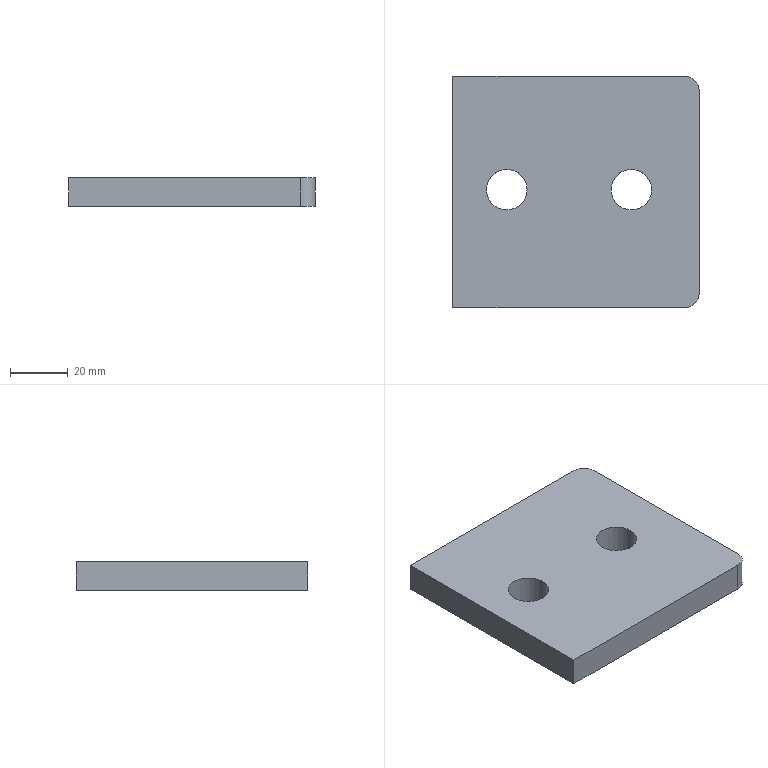Part | SolidWorks | features Extrusion 1, HoleWzd 1 | 1 solid | 12 faces | box 85 x 80 x 10 mm | volume 64814 mm3 | cylinder 6 | plane 6 | commonest cylinder face diameters 14 x4 10 x2
STEP:
#1=CARTESIAN_POINT('',(12.1,0.8,0.));
#2=VERTEX_POINT('',#1);
#3=CARTESIAN_POINT('',(26.1,0.8,0.));
#4=VERTEX_POINT('',#3);
#5=CARTESIAN_POINT('',(19.1,0.8,0.));
#6=DIRECTION('',(0.,0.,1.));
#7=DIRECTION('',(1.,0.,0.));
#8=AXIS2_PLACEMENT_3D('',#5,#6,#7);
#9=CIRCLE('',#8,7.);
#10=EDGE_CURVE('',#2,#4,#9,.T.);
#11=ORIENTED_EDGE('',*,*,#10,.F.);
#12=CARTESIAN_POINT('',(12.1,0.8,10.));
#13=VERTEX_POINT('',#12);
#14=CARTESIAN_POINT('',(12.1,0.8,10.));
#15=DIRECTION('',(0.,0.,1.));
#16=VECTOR('',#15,1000.);
#17=LINE('',#14,#16);
#18=EDGE_CURVE('',#2,#13,#17,.T.);
#19=ORIENTED_EDGE('',*,*,#18,.T.);
#20=CARTESIAN_POINT('',(26.1,0.8,10.));
#21=VERTEX_POINT('',#20);
#22=CARTESIAN_POINT('',(19.1,0.8,10.));
#23=DIRECTION('',(0.,0.,1.));
#24=DIRECTION('',(1.,0.,0.));
#25=AXIS2_PLACEMENT_3D('',#22,#23,#24);
#26=CIRCLE('',#25,7.);
#27=EDGE_CURVE('',#13,#21,#26,.T.);
#28=ORIENTED_EDGE('',*,*,#27,.T.);
#29=CARTESIAN_POINT('',(26.1,0.8,10.));
#30=DIRECTION('',(0.,0.,1.));
#31=VECTOR('',#30,1000.);
#32=LINE('',#29,#31);
#33=EDGE_CURVE('',#4,#21,#32,.T.);
#34=ORIENTED_EDGE('',*,*,#33,.F.);
#35=EDGE_LOOP('',(#11,#19,#28,#34));
#36=FACE_OUTER_BOUND('',#35,.T.);
#37=CARTESIAN_POINT('',(19.1,0.8,10.));
#38=DIRECTION('',(0.,0.,1.));
#39=DIRECTION('',(1.,0.,0.));
#40=AXIS2_PLACEMENT_3D('',#37,#38,#39);
#41=CYLINDRICAL_SURFACE('',#40,7.);
#42=ADVANCED_FACE('',(#36),#41,.F.);
#43=CARTESIAN_POINT('',(-30.9,0.8,0.));
#44=VERTEX_POINT('',#43);
#45=CARTESIAN_POINT('',(-16.9,0.8,0.));
#46=VERTEX_POINT('',#45);
#47=CARTESIAN_POINT('',(-23.9,0.8,0.));
#48=DIRECTION('',(0.,0.,1.));
#49=DIRECTION('',(1.,0.,0.));
#50=AXIS2_PLACEMENT_3D('',#47,#48,#49);
#51=CIRCLE('',#50,7.);
#52=EDGE_CURVE('',#44,#46,#51,.T.);
#53=ORIENTED_EDGE('',*,*,#52,.F.);
#54=CARTESIAN_POINT('',(-30.9,0.8,10.));
#55=VERTEX_POINT('',#54);
#56=CARTESIAN_POINT('',(-30.9,0.8,10.));
#57=DIRECTION('',(0.,0.,1.));
#58=VECTOR('',#57,1000.);
#59=LINE('',#56,#58);
#60=EDGE_CURVE('',#44,#55,#59,.T.);
#61=ORIENTED_EDGE('',*,*,#60,.T.);
#62=CARTESIAN_POINT('',(-16.9,0.8,10.));
#63=VERTEX_POINT('',#62);
#64=CARTESIAN_POINT('',(-23.9,0.8,10.));
#65=DIRECTION('',(0.,0.,1.));
#66=DIRECTION('',(1.,0.,0.));
#67=AXIS2_PLACEMENT_3D('',#64,#65,#66);
#68=CIRCLE('',#67,7.);
#69=EDGE_CURVE('',#55,#63,#68,.T.);
#70=ORIENTED_EDGE('',*,*,#69,.T.);
#71=CARTESIAN_POINT('',(-16.9,0.8,10.));
#72=DIRECTION('',(0.,0.,1.));
#73=VECTOR('',#72,1000.);
#74=LINE('',#71,#73);
#75=EDGE_CURVE('',#46,#63,#74,.T.);
#76=ORIENTED_EDGE('',*,*,#75,.F.);
#77=EDGE_LOOP('',(#53,#61,#70,#76));
#78=FACE_OUTER_BOUND('',#77,.T.);
#79=CARTESIAN_POINT('',(-23.9,0.8,10.));
#80=DIRECTION('',(0.,0.,1.));
#81=DIRECTION('',(1.,0.,0.));
#82=AXIS2_PLACEMENT_3D('',#79,#80,#81);
#83=CYLINDRICAL_SURFACE('',#82,7.);
#84=ADVANCED_FACE('',(#78),#83,.F.);
#85=CARTESIAN_POINT('',(-42.5,40.,0.));
#86=VERTEX_POINT('',#85);
#87=CARTESIAN_POINT('',(-42.5,-40.,0.));
#88=VERTEX_POINT('',#87);
#89=CARTESIAN_POINT('',(-42.5,40.,0.));
#90=DIRECTION('',(0.,-1.,0.));
#91=VECTOR('',#90,1000.);
#92=LINE('',#89,#91);
#93=EDGE_CURVE('',#86,#88,#92,.T.);
#94=ORIENTED_EDGE('',*,*,#93,.T.);
#95=CARTESIAN_POINT('',(-42.5,-40.,10.));
#96=VERTEX_POINT('',#95);
#97=CARTESIAN_POINT('',(-42.5,-40.,10.));
#98=DIRECTION('',(0.,0.,-1.));
#99=VECTOR('',#98,1000.);
#100=LINE('',#97,#99);
#101=EDGE_CURVE('',#96,#88,#100,.T.);
#102=ORIENTED_EDGE('',*,*,#101,.F.);
#103=CARTESIAN_POINT('',(-42.5,40.,10.));
#104=VERTEX_POINT('',#103);
#105=CARTESIAN_POINT('',(-42.5,40.,10.));
#106=DIRECTION('',(0.,-1.,0.));
#107=VECTOR('',#106,1000.);
#108=LINE('',#105,#107);
#109=EDGE_CURVE('',#104,#96,#108,.T.);
#110=ORIENTED_EDGE('',*,*,#109,.F.);
#111=CARTESIAN_POINT('',(-42.5,40.,10.));
#112=DIRECTION('',(0.,0.,-1.));
#113=VECTOR('',#112,1000.);
#114=LINE('',#111,#113);
#115=EDGE_CURVE('',#104,#86,#114,.T.);
#116=ORIENTED_EDGE('',*,*,#115,.T.);
#117=EDGE_LOOP('',(#94,#102,#110,#116));
#118=FACE_OUTER_BOUND('',#117,.T.);
#119=CARTESIAN_POINT('',(-42.5,40.,10.));
#120=DIRECTION('',(1.,0.,0.));
#121=DIRECTION('',(0.,1.,0.));
#122=AXIS2_PLACEMENT_3D('',#119,#120,#121);
#123=PLANE('',#122);
#124=ADVANCED_FACE('',(#118),#123,.F.);
#125=CARTESIAN_POINT('',(37.5,-40.,0.));
#126=VERTEX_POINT('',#125);
#127=CARTESIAN_POINT('',(-42.5,-40.,0.));
#128=DIRECTION('',(1.,0.,0.));
#129=VECTOR('',#128,1000.);
#130=LINE('',#127,#129);
#131=EDGE_CURVE('',#88,#126,#130,.T.);
#132=ORIENTED_EDGE('',*,*,#131,.T.);
#133=CARTESIAN_POINT('',(37.5,-40.,10.));
#134=VERTEX_POINT('',#133);
#135=CARTESIAN_POINT('',(37.5,-40.,10.));
#136=DIRECTION('',(0.,0.,-1.));
#137=VECTOR('',#136,1000.);
#138=LINE('',#135,#137);
#139=EDGE_CURVE('',#134,#126,#138,.T.);
#140=ORIENTED_EDGE('',*,*,#139,.F.);
#141=CARTESIAN_POINT('',(-42.5,-40.,10.));
#142=DIRECTION('',(1.,0.,0.));
#143=VECTOR('',#142,1000.);
#144=LINE('',#141,#143);
#145=EDGE_CURVE('',#96,#134,#144,.T.);
#146=ORIENTED_EDGE('',*,*,#145,.F.);
#147=ORIENTED_EDGE('',*,*,#101,.T.);
#148=EDGE_LOOP('',(#132,#140,#146,#147));
#149=FACE_OUTER_BOUND('',#148,.T.);
#150=CARTESIAN_POINT('',(-42.5,-40.,10.));
#151=DIRECTION('',(0.,1.,0.));
#152=DIRECTION('',(0.,0.,1.));
#153=AXIS2_PLACEMENT_3D('',#150,#151,#152);
#154=PLANE('',#153);
#155=ADVANCED_FACE('',(#149),#154,.F.);
#156=CARTESIAN_POINT('',(42.5,-35.,0.));
#157=VERTEX_POINT('',#156);
#158=CARTESIAN_POINT('',(37.5,-35.,0.));
#159=DIRECTION('',(0.,0.,1.));
#160=DIRECTION('',(1.,0.,0.));
#161=AXIS2_PLACEMENT_3D('',#158,#159,#160);
#162=CIRCLE('',#161,5.);
#163=EDGE_CURVE('',#126,#157,#162,.T.);
#164=ORIENTED_EDGE('',*,*,#163,.T.);
#165=CARTESIAN_POINT('',(42.5,-35.,10.));
#166=VERTEX_POINT('',#165);
#167=CARTESIAN_POINT('',(42.5,-35.,10.));
#168=DIRECTION('',(0.,0.,-1.));
#169=VECTOR('',#168,1000.);
#170=LINE('',#167,#169);
#171=EDGE_CURVE('',#166,#157,#170,.T.);
#172=ORIENTED_EDGE('',*,*,#171,.F.);
#173=CARTESIAN_POINT('',(37.5,-35.,10.));
#174=DIRECTION('',(0.,0.,1.));
#175=DIRECTION('',(1.,0.,0.));
#176=AXIS2_PLACEMENT_3D('',#173,#174,#175);
#177=CIRCLE('',#176,5.);
#178=EDGE_CURVE('',#134,#166,#177,.T.);
#179=ORIENTED_EDGE('',*,*,#178,.F.);
#180=ORIENTED_EDGE('',*,*,#139,.T.);
#181=EDGE_LOOP('',(#164,#172,#179,#180));
#182=FACE_OUTER_BOUND('',#181,.T.);
#183=CARTESIAN_POINT('',(37.5,-35.,10.));
#184=DIRECTION('',(0.,0.,-1.));
#185=DIRECTION('',(-1.,0.,0.));
#186=AXIS2_PLACEMENT_3D('',#183,#184,#185);
#187=CYLINDRICAL_SURFACE('',#186,5.);
#188=ADVANCED_FACE('',(#182),#187,.T.);
#189=CARTESIAN_POINT('',(42.5,35.,0.));
#190=VERTEX_POINT('',#189);
#191=CARTESIAN_POINT('',(42.5,35.,0.));
#192=DIRECTION('',(0.,1.,0.));
#193=VECTOR('',#192,1000.);
#194=LINE('',#191,#193);
#195=EDGE_CURVE('',#157,#190,#194,.T.);
#196=ORIENTED_EDGE('',*,*,#195,.T.);
#197=CARTESIAN_POINT('',(42.5,35.,10.));
#198=VERTEX_POINT('',#197);
#199=CARTESIAN_POINT('',(42.5,35.,10.));
#200=DIRECTION('',(0.,0.,-1.));
#201=VECTOR('',#200,1000.);
#202=LINE('',#199,#201);
#203=EDGE_CURVE('',#198,#190,#202,.T.);
#204=ORIENTED_EDGE('',*,*,#203,.F.);
#205=CARTESIAN_POINT('',(42.5,35.,10.));
#206=DIRECTION('',(0.,1.,0.));
#207=VECTOR('',#206,1000.);
#208=LINE('',#205,#207);
#209=EDGE_CURVE('',#166,#198,#208,.T.);
#210=ORIENTED_EDGE('',*,*,#209,.F.);
#211=ORIENTED_EDGE('',*,*,#171,.T.);
#212=EDGE_LOOP('',(#196,#204,#210,#211));
#213=FACE_OUTER_BOUND('',#212,.T.);
#214=CARTESIAN_POINT('',(42.5,35.,10.));
#215=DIRECTION('',(-1.,0.,0.));
#216=DIRECTION('',(0.,0.,1.));
#217=AXIS2_PLACEMENT_3D('',#214,#215,#216);
#218=PLANE('',#217);
#219=ADVANCED_FACE('',(#213),#218,.F.);
#220=CARTESIAN_POINT('',(37.5,40.,0.));
#221=VERTEX_POINT('',#220);
#222=CARTESIAN_POINT('',(37.5,35.,0.));
#223=DIRECTION('',(0.,0.,1.));
#224=DIRECTION('',(-1.,0.,0.));
#225=AXIS2_PLACEMENT_3D('',#222,#223,#224);
#226=CIRCLE('',#225,5.);
#227=EDGE_CURVE('',#190,#221,#226,.T.);
#228=ORIENTED_EDGE('',*,*,#227,.T.);
#229=CARTESIAN_POINT('',(37.5,40.,10.));
#230=VERTEX_POINT('',#229);
#231=CARTESIAN_POINT('',(37.5,40.,10.));
#232=DIRECTION('',(0.,0.,-1.));
#233=VECTOR('',#232,1000.);
#234=LINE('',#231,#233);
#235=EDGE_CURVE('',#230,#221,#234,.T.);
#236=ORIENTED_EDGE('',*,*,#235,.F.);
#237=CARTESIAN_POINT('',(37.5,35.,10.));
#238=DIRECTION('',(0.,0.,1.));
#239=DIRECTION('',(-1.,0.,0.));
#240=AXIS2_PLACEMENT_3D('',#237,#238,#239);
#241=CIRCLE('',#240,5.);
#242=EDGE_CURVE('',#198,#230,#241,.T.);
#243=ORIENTED_EDGE('',*,*,#242,.F.);
#244=ORIENTED_EDGE('',*,*,#203,.T.);
#245=EDGE_LOOP('',(#228,#236,#243,#244));
#246=FACE_OUTER_BOUND('',#245,.T.);
#247=CARTESIAN_POINT('',(37.5,35.,10.));
#248=DIRECTION('',(0.,0.,-1.));
#249=DIRECTION('',(-1.,0.,0.));
#250=AXIS2_PLACEMENT_3D('',#247,#248,#249);
#251=CYLINDRICAL_SURFACE('',#250,5.);
#252=ADVANCED_FACE('',(#246),#251,.T.);
#253=CARTESIAN_POINT('',(-42.5,40.,0.));
#254=DIRECTION('',(-1.,0.,0.));
#255=VECTOR('',#254,1000.);
#256=LINE('',#253,#255);
#257=EDGE_CURVE('',#221,#86,#256,.T.);
#258=ORIENTED_EDGE('',*,*,#257,.T.);
#259=ORIENTED_EDGE('',*,*,#115,.F.);
#260=CARTESIAN_POINT('',(-42.5,40.,10.));
#261=DIRECTION('',(-1.,0.,0.));
#262=VECTOR('',#261,1000.);
#263=LINE('',#260,#262);
#264=EDGE_CURVE('',#230,#104,#263,.T.);
#265=ORIENTED_EDGE('',*,*,#264,.F.);
#266=ORIENTED_EDGE('',*,*,#235,.T.);
#267=EDGE_LOOP('',(#258,#259,#265,#266));
#268=FACE_OUTER_BOUND('',#267,.T.);
#269=CARTESIAN_POINT('',(-42.5,40.,10.));
#270=DIRECTION('',(0.,-1.,0.));
#271=DIRECTION('',(0.,0.,-1.));
#272=AXIS2_PLACEMENT_3D('',#269,#270,#271);
#273=PLANE('',#272);
#274=ADVANCED_FACE('',(#268),#273,.F.);
#275=CARTESIAN_POINT('',(19.1,0.8,10.));
#276=DIRECTION('',(0.,0.,1.));
#277=DIRECTION('',(1.,0.,0.));
#278=AXIS2_PLACEMENT_3D('',#275,#276,#277);
#279=CIRCLE('',#278,7.);
#280=EDGE_CURVE('',#21,#13,#279,.T.);
#281=ORIENTED_EDGE('',*,*,#280,.F.);
#282=ORIENTED_EDGE('',*,*,#27,.F.);
#283=EDGE_LOOP('',(#281,#282));
#284=FACE_BOUND('',#283,.T.);
#285=CARTESIAN_POINT('',(-23.9,0.8,10.));
#286=DIRECTION('',(0.,0.,1.));
#287=DIRECTION('',(1.,0.,0.));
#288=AXIS2_PLACEMENT_3D('',#285,#286,#287);
#289=CIRCLE('',#288,7.);
#290=EDGE_CURVE('',#63,#55,#289,.T.);
#291=ORIENTED_EDGE('',*,*,#290,.F.);
#292=ORIENTED_EDGE('',*,*,#69,.F.);
#293=EDGE_LOOP('',(#291,#292));
#294=FACE_BOUND('',#293,.T.);
#295=ORIENTED_EDGE('',*,*,#109,.T.);
#296=ORIENTED_EDGE('',*,*,#145,.T.);
#297=ORIENTED_EDGE('',*,*,#178,.T.);
#298=ORIENTED_EDGE('',*,*,#209,.T.);
#299=ORIENTED_EDGE('',*,*,#242,.T.);
#300=ORIENTED_EDGE('',*,*,#264,.T.);
#301=EDGE_LOOP('',(#295,#296,#297,#298,#299,#300));
#302=FACE_OUTER_BOUND('',#301,.T.);
#303=CARTESIAN_POINT('',(37.5,-35.,10.));
#304=DIRECTION('',(0.,0.,1.));
#305=DIRECTION('',(1.,0.,0.));
#306=AXIS2_PLACEMENT_3D('',#303,#304,#305);
#307=PLANE('',#306);
#308=ADVANCED_FACE('',(#284,#294,#302),#307,.T.);
#309=CARTESIAN_POINT('',(19.1,0.8,0.));
#310=DIRECTION('',(0.,0.,1.));
#311=DIRECTION('',(1.,0.,0.));
#312=AXIS2_PLACEMENT_3D('',#309,#310,#311);
#313=CIRCLE('',#312,7.);
#314=EDGE_CURVE('',#4,#2,#313,.T.);
#315=ORIENTED_EDGE('',*,*,#314,.T.);
#316=ORIENTED_EDGE('',*,*,#10,.T.);
#317=EDGE_LOOP('',(#315,#316));
#318=FACE_BOUND('',#317,.T.);
#319=CARTESIAN_POINT('',(-23.9,0.8,0.));
#320=DIRECTION('',(0.,0.,1.));
#321=DIRECTION('',(1.,0.,0.));
#322=AXIS2_PLACEMENT_3D('',#319,#320,#321);
#323=CIRCLE('',#322,7.);
#324=EDGE_CURVE('',#46,#44,#323,.T.);
#325=ORIENTED_EDGE('',*,*,#324,.T.);
#326=ORIENTED_EDGE('',*,*,#52,.T.);
#327=EDGE_LOOP('',(#325,#326));
#328=FACE_BOUND('',#327,.T.);
#329=ORIENTED_EDGE('',*,*,#93,.F.);
#330=ORIENTED_EDGE('',*,*,#257,.F.);
#331=ORIENTED_EDGE('',*,*,#227,.F.);
#332=ORIENTED_EDGE('',*,*,#195,.F.);
#333=ORIENTED_EDGE('',*,*,#163,.F.);
#334=ORIENTED_EDGE('',*,*,#131,.F.);
#335=EDGE_LOOP('',(#329,#330,#331,#332,#333,#334));
#336=FACE_OUTER_BOUND('',#335,.T.);
#337=CARTESIAN_POINT('',(37.5,-35.,0.));
#338=DIRECTION('',(0.,0.,1.));
#339=DIRECTION('',(1.,0.,0.));
#340=AXIS2_PLACEMENT_3D('',#337,#338,#339);
#341=PLANE('',#340);
#342=ADVANCED_FACE('',(#318,#328,#336),#341,.F.);
#343=ORIENTED_EDGE('',*,*,#60,.F.);
#344=ORIENTED_EDGE('',*,*,#324,.F.);
#345=ORIENTED_EDGE('',*,*,#75,.T.);
#346=ORIENTED_EDGE('',*,*,#290,.T.);
#347=EDGE_LOOP('',(#343,#344,#345,#346));
#348=FACE_OUTER_BOUND('',#347,.T.);
#349=CARTESIAN_POINT('',(-23.9,0.8,10.));
#350=DIRECTION('',(0.,0.,1.));
#351=DIRECTION('',(1.,0.,0.));
#352=AXIS2_PLACEMENT_3D('',#349,#350,#351);
#353=CYLINDRICAL_SURFACE('',#352,7.);
#354=ADVANCED_FACE('',(#348),#353,.F.);
#355=ORIENTED_EDGE('',*,*,#18,.F.);
#356=ORIENTED_EDGE('',*,*,#314,.F.);
#357=ORIENTED_EDGE('',*,*,#33,.T.);
#358=ORIENTED_EDGE('',*,*,#280,.T.);
#359=EDGE_LOOP('',(#355,#356,#357,#358));
#360=FACE_OUTER_BOUND('',#359,.T.);
#361=CARTESIAN_POINT('',(19.1,0.8,10.));
#362=DIRECTION('',(0.,0.,1.));
#363=DIRECTION('',(1.,0.,0.));
#364=AXIS2_PLACEMENT_3D('',#361,#362,#363);
#365=CYLINDRICAL_SURFACE('',#364,7.);
#366=ADVANCED_FACE('',(#360),#365,.F.);
#367=CLOSED_SHELL('',(#42,#84,#124,#155,#188,#219,#252,#274,#308,#342,#354,#366));
#368=MANIFOLD_SOLID_BREP('',#367);
#369=CARTESIAN_POINT('',(0.,0.,0.));
#370=DIRECTION('',(0.,0.,1.));
#371=DIRECTION('',(1.,0.,0.));
#372=AXIS2_PLACEMENT_3D('',#369,#370,#371);
#373=(LENGTH_UNIT()NAMED_UNIT(*)SI_UNIT(.MILLI.,.METRE.));
#374=UNCERTAINTY_MEASURE_WITH_UNIT(LENGTH_MEASURE(0.00001),#373,'','');
#375=(NAMED_UNIT(*)PLANE_ANGLE_UNIT()SI_UNIT($,.RADIAN.));
#376=(NAMED_UNIT(*)SI_UNIT($,.STERADIAN.)SOLID_ANGLE_UNIT());
#377=(GEOMETRIC_REPRESENTATION_CONTEXT(3)GLOBAL_UNCERTAINTY_ASSIGNED_CONTEXT((#374))GLOBAL_UNIT_ASSIGNED_CONTEXT((#373,#375,#376))REPRESENTATION_CONTEXT('',''));
#378=ADVANCED_BREP_SHAPE_REPRESENTATION('',(#368,#372),#377);